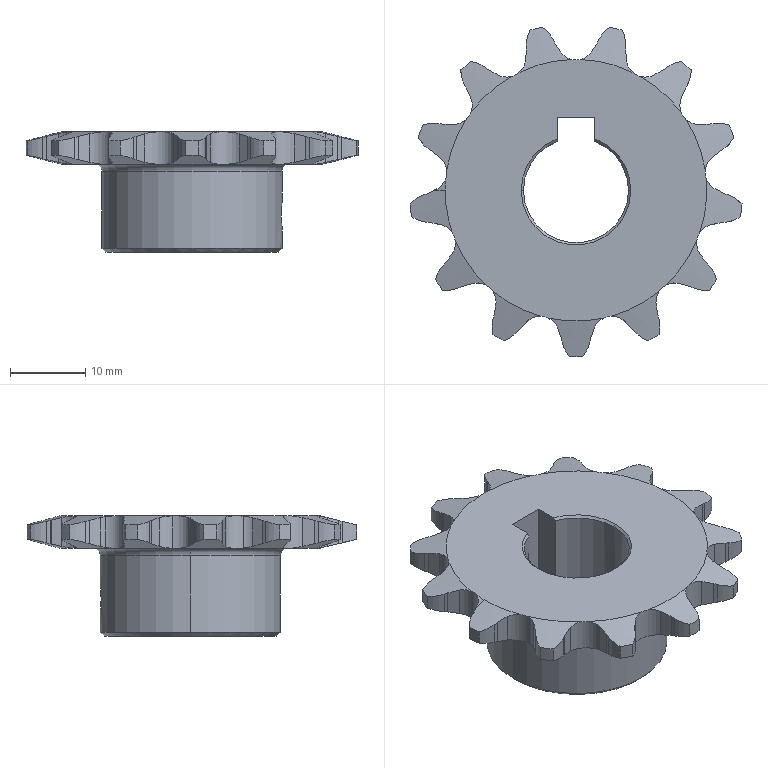Part | STEP file | Drive sprocket 06B-13 teeth_bore φ14 | 1 solid | 164 faces | box 44.21 x 43.904 x 16.003 mm | volume 7455 mm3 | cylinder 94 | cone 36 | plane 32 | torus 2 | commonest cylinder face diameters 8.57 x28 13.236 x27 5.108 x17 44.359 x13 3.3 x4 14 x3